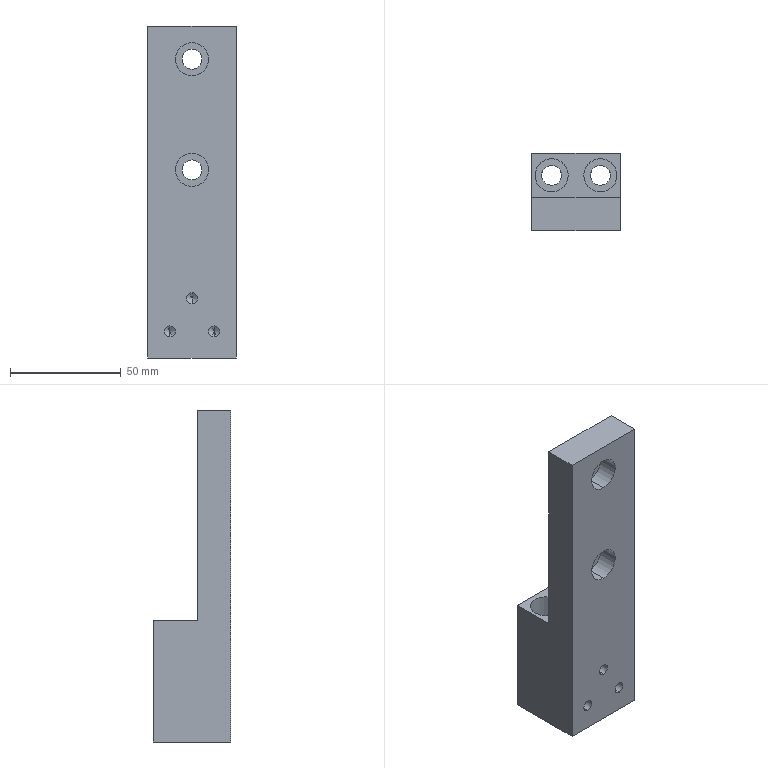Part | SolidWorks | features BaseBody 1 | 1 solid | 52 faces | box 40 x 35 x 150 mm | volume 115005 mm3 | cylinder 28 | cone 12 | plane 12 | commonest cylinder face diameters 9 x8 15 x8 5 x6 6.8 x6
STEP:
#1=CARTESIAN_POINT('',(0.,17.,-45.5));
#2=VERTEX_POINT('',#1);
#3=CARTESIAN_POINT('',(0.,17.,-50.5));
#4=VERTEX_POINT('',#3);
#5=CARTESIAN_POINT('',(0.,17.,-48.));
#6=DIRECTION('',(0.,-1.,0.));
#7=DIRECTION('',(0.,0.,-1.));
#8=AXIS2_PLACEMENT_3D('',#5,#6,#7);
#9=CIRCLE('',#8,2.5);
#10=EDGE_CURVE('',#2,#4,#9,.T.);
#11=ORIENTED_EDGE('',*,*,#10,.F.);
#12=CARTESIAN_POINT('',(0.,0.,-45.5));
#13=VERTEX_POINT('',#12);
#14=CARTESIAN_POINT('',(0.,0.,-45.5));
#15=DIRECTION('',(0.,-1.,0.));
#16=VECTOR('',#15,1000.);
#17=LINE('',#14,#16);
#18=EDGE_CURVE('',#2,#13,#17,.T.);
#19=ORIENTED_EDGE('',*,*,#18,.T.);
#20=CARTESIAN_POINT('',(0.,0.,-50.5));
#21=VERTEX_POINT('',#20);
#22=CARTESIAN_POINT('',(0.,0.,-48.));
#23=DIRECTION('',(0.,-1.,0.));
#24=DIRECTION('',(0.,0.,-1.));
#25=AXIS2_PLACEMENT_3D('',#22,#23,#24);
#26=CIRCLE('',#25,2.5);
#27=EDGE_CURVE('',#13,#21,#26,.T.);
#28=ORIENTED_EDGE('',*,*,#27,.T.);
#29=CARTESIAN_POINT('',(0.,0.,-50.5));
#30=DIRECTION('',(0.,-1.,0.));
#31=VECTOR('',#30,1000.);
#32=LINE('',#29,#31);
#33=EDGE_CURVE('',#4,#21,#32,.T.);
#34=ORIENTED_EDGE('',*,*,#33,.F.);
#35=EDGE_LOOP('',(#11,#19,#28,#34));
#36=FACE_OUTER_BOUND('',#35,.T.);
#37=CARTESIAN_POINT('',(0.,0.,-48.));
#38=DIRECTION('',(0.,-1.,0.));
#39=DIRECTION('',(0.,0.,-1.));
#40=AXIS2_PLACEMENT_3D('',#37,#38,#39);
#41=CYLINDRICAL_SURFACE('',#40,2.5);
#42=ADVANCED_FACE('',(#36),#41,.F.);
#43=CARTESIAN_POINT('',(0.,18.502,-48.));
#44=VERTEX_POINT('',#43);
#45=CARTESIAN_POINT('',(0.,17.,-50.5));
#46=DIRECTION('',(0.,-0.515,-0.8572));
#47=VECTOR('',#46,1000.);
#48=LINE('',#45,#47);
#49=EDGE_CURVE('',#44,#4,#48,.T.);
#50=ORIENTED_EDGE('',*,*,#49,.F.);
#51=CARTESIAN_POINT('',(0.,17.,-45.5));
#52=DIRECTION('',(0.,-0.515,0.8572));
#53=VECTOR('',#52,1000.);
#54=LINE('',#51,#53);
#55=EDGE_CURVE('',#44,#2,#54,.T.);
#56=ORIENTED_EDGE('',*,*,#55,.T.);
#57=ORIENTED_EDGE('',*,*,#10,.T.);
#58=EDGE_LOOP('',(#50,#56,#57));
#59=FACE_OUTER_BOUND('',#58,.T.);
#60=CARTESIAN_POINT('',(0.,17.,-48.));
#61=DIRECTION('',(0.,-1.,0.));
#62=DIRECTION('',(0.,0.,-1.));
#63=AXIS2_PLACEMENT_3D('',#60,#61,#62);
#64=CONICAL_SURFACE('',#63,2.5,1.03);
#65=ADVANCED_FACE('',(#59),#64,.F.);
#66=CARTESIAN_POINT('',(-10.,17.,-60.5));
#67=VERTEX_POINT('',#66);
#68=CARTESIAN_POINT('',(-10.,17.,-65.5));
#69=VERTEX_POINT('',#68);
#70=CARTESIAN_POINT('',(-10.,17.,-63.));
#71=DIRECTION('',(0.,-1.,0.));
#72=DIRECTION('',(0.,0.,-1.));
#73=AXIS2_PLACEMENT_3D('',#70,#71,#72);
#74=CIRCLE('',#73,2.5);
#75=EDGE_CURVE('',#67,#69,#74,.T.);
#76=ORIENTED_EDGE('',*,*,#75,.F.);
#77=CARTESIAN_POINT('',(-10.,0.,-60.5));
#78=VERTEX_POINT('',#77);
#79=CARTESIAN_POINT('',(-10.,0.,-60.5));
#80=DIRECTION('',(0.,-1.,0.));
#81=VECTOR('',#80,1000.);
#82=LINE('',#79,#81);
#83=EDGE_CURVE('',#67,#78,#82,.T.);
#84=ORIENTED_EDGE('',*,*,#83,.T.);
#85=CARTESIAN_POINT('',(-10.,0.,-65.5));
#86=VERTEX_POINT('',#85);
#87=CARTESIAN_POINT('',(-10.,0.,-63.));
#88=DIRECTION('',(0.,-1.,0.));
#89=DIRECTION('',(0.,0.,-1.));
#90=AXIS2_PLACEMENT_3D('',#87,#88,#89);
#91=CIRCLE('',#90,2.5);
#92=EDGE_CURVE('',#78,#86,#91,.T.);
#93=ORIENTED_EDGE('',*,*,#92,.T.);
#94=CARTESIAN_POINT('',(-10.,0.,-65.5));
#95=DIRECTION('',(0.,-1.,0.));
#96=VECTOR('',#95,1000.);
#97=LINE('',#94,#96);
#98=EDGE_CURVE('',#69,#86,#97,.T.);
#99=ORIENTED_EDGE('',*,*,#98,.F.);
#100=EDGE_LOOP('',(#76,#84,#93,#99));
#101=FACE_OUTER_BOUND('',#100,.T.);
#102=CARTESIAN_POINT('',(-10.,0.,-63.));
#103=DIRECTION('',(0.,-1.,0.));
#104=DIRECTION('',(0.,0.,-1.));
#105=AXIS2_PLACEMENT_3D('',#102,#103,#104);
#106=CYLINDRICAL_SURFACE('',#105,2.5);
#107=ADVANCED_FACE('',(#101),#106,.F.);
#108=CARTESIAN_POINT('',(-10.,18.502,-63.));
#109=VERTEX_POINT('',#108);
#110=CARTESIAN_POINT('',(-10.,17.,-65.5));
#111=DIRECTION('',(0.,-0.515,-0.8572));
#112=VECTOR('',#111,1000.);
#113=LINE('',#110,#112);
#114=EDGE_CURVE('',#109,#69,#113,.T.);
#115=ORIENTED_EDGE('',*,*,#114,.F.);
#116=CARTESIAN_POINT('',(-10.,17.,-60.5));
#117=DIRECTION('',(0.,-0.515,0.8572));
#118=VECTOR('',#117,1000.);
#119=LINE('',#116,#118);
#120=EDGE_CURVE('',#109,#67,#119,.T.);
#121=ORIENTED_EDGE('',*,*,#120,.T.);
#122=ORIENTED_EDGE('',*,*,#75,.T.);
#123=EDGE_LOOP('',(#115,#121,#122));
#124=FACE_OUTER_BOUND('',#123,.T.);
#125=CARTESIAN_POINT('',(-10.,17.,-63.));
#126=DIRECTION('',(0.,-1.,0.));
#127=DIRECTION('',(0.,0.,-1.));
#128=AXIS2_PLACEMENT_3D('',#125,#126,#127);
#129=CONICAL_SURFACE('',#128,2.5,1.03);
#130=ADVANCED_FACE('',(#124),#129,.F.);
#131=CARTESIAN_POINT('',(10.,17.,-60.5));
#132=VERTEX_POINT('',#131);
#133=CARTESIAN_POINT('',(10.,17.,-65.5));
#134=VERTEX_POINT('',#133);
#135=CARTESIAN_POINT('',(10.,17.,-63.));
#136=DIRECTION('',(0.,-1.,0.));
#137=DIRECTION('',(0.,0.,-1.));
#138=AXIS2_PLACEMENT_3D('',#135,#136,#137);
#139=CIRCLE('',#138,2.5);
#140=EDGE_CURVE('',#132,#134,#139,.T.);
#141=ORIENTED_EDGE('',*,*,#140,.F.);
#142=CARTESIAN_POINT('',(10.,0.,-60.5));
#143=VERTEX_POINT('',#142);
#144=CARTESIAN_POINT('',(10.,0.,-60.5));
#145=DIRECTION('',(0.,-1.,0.));
#146=VECTOR('',#145,1000.);
#147=LINE('',#144,#146);
#148=EDGE_CURVE('',#132,#143,#147,.T.);
#149=ORIENTED_EDGE('',*,*,#148,.T.);
#150=CARTESIAN_POINT('',(10.,0.,-65.5));
#151=VERTEX_POINT('',#150);
#152=CARTESIAN_POINT('',(10.,0.,-63.));
#153=DIRECTION('',(0.,-1.,0.));
#154=DIRECTION('',(0.,0.,-1.));
#155=AXIS2_PLACEMENT_3D('',#152,#153,#154);
#156=CIRCLE('',#155,2.5);
#157=EDGE_CURVE('',#143,#151,#156,.T.);
#158=ORIENTED_EDGE('',*,*,#157,.T.);
#159=CARTESIAN_POINT('',(10.,0.,-65.5));
#160=DIRECTION('',(0.,-1.,0.));
#161=VECTOR('',#160,1000.);
#162=LINE('',#159,#161);
#163=EDGE_CURVE('',#134,#151,#162,.T.);
#164=ORIENTED_EDGE('',*,*,#163,.F.);
#165=EDGE_LOOP('',(#141,#149,#158,#164));
#166=FACE_OUTER_BOUND('',#165,.T.);
#167=CARTESIAN_POINT('',(10.,0.,-63.));
#168=DIRECTION('',(0.,-1.,0.));
#169=DIRECTION('',(0.,0.,-1.));
#170=AXIS2_PLACEMENT_3D('',#167,#168,#169);
#171=CYLINDRICAL_SURFACE('',#170,2.5);
#172=ADVANCED_FACE('',(#166),#171,.F.);
#173=CARTESIAN_POINT('',(10.,18.502,-63.));
#174=VERTEX_POINT('',#173);
#175=CARTESIAN_POINT('',(10.,17.,-65.5));
#176=DIRECTION('',(0.,-0.515,-0.8572));
#177=VECTOR('',#176,1000.);
#178=LINE('',#175,#177);
#179=EDGE_CURVE('',#174,#134,#178,.T.);
#180=ORIENTED_EDGE('',*,*,#179,.F.);
#181=CARTESIAN_POINT('',(10.,17.,-60.5));
#182=DIRECTION('',(0.,-0.515,0.8572));
#183=VECTOR('',#182,1000.);
#184=LINE('',#181,#183);
#185=EDGE_CURVE('',#174,#132,#184,.T.);
#186=ORIENTED_EDGE('',*,*,#185,.T.);
#187=ORIENTED_EDGE('',*,*,#140,.T.);
#188=EDGE_LOOP('',(#180,#186,#187));
#189=FACE_OUTER_BOUND('',#188,.T.);
#190=CARTESIAN_POINT('',(10.,17.,-63.));
#191=DIRECTION('',(0.,-1.,0.));
#192=DIRECTION('',(0.,0.,-1.));
#193=AXIS2_PLACEMENT_3D('',#190,#191,#192);
#194=CONICAL_SURFACE('',#193,2.5,1.03);
#195=ADVANCED_FACE('',(#189),#194,.F.);
#196=CARTESIAN_POINT('',(-2.25,7.5,-51.6));
#197=VERTEX_POINT('',#196);
#198=CARTESIAN_POINT('',(-2.25,7.5,-58.4));
#199=VERTEX_POINT('',#198);
#200=CARTESIAN_POINT('',(-2.25,7.5,-55.));
#201=DIRECTION('',(1.,0.,0.));
#202=DIRECTION('',(0.,0.,-1.));
#203=AXIS2_PLACEMENT_3D('',#200,#201,#202);
#204=CIRCLE('',#203,3.4);
#205=EDGE_CURVE('',#197,#199,#204,.T.);
#206=ORIENTED_EDGE('',*,*,#205,.F.);
#207=CARTESIAN_POINT('',(20.,7.5,-51.6));
#208=VERTEX_POINT('',#207);
#209=CARTESIAN_POINT('',(20.,7.5,-51.6));
#210=DIRECTION('',(1.,0.,0.));
#211=VECTOR('',#210,1000.);
#212=LINE('',#209,#211);
#213=EDGE_CURVE('',#197,#208,#212,.T.);
#214=ORIENTED_EDGE('',*,*,#213,.T.);
#215=CARTESIAN_POINT('',(20.,7.5,-58.4));
#216=VERTEX_POINT('',#215);
#217=CARTESIAN_POINT('',(20.,7.5,-55.));
#218=DIRECTION('',(1.,0.,0.));
#219=DIRECTION('',(0.,0.,-1.));
#220=AXIS2_PLACEMENT_3D('',#217,#218,#219);
#221=CIRCLE('',#220,3.4);
#222=EDGE_CURVE('',#208,#216,#221,.T.);
#223=ORIENTED_EDGE('',*,*,#222,.T.);
#224=CARTESIAN_POINT('',(20.,7.5,-58.4));
#225=DIRECTION('',(1.,0.,0.));
#226=VECTOR('',#225,1000.);
#227=LINE('',#224,#226);
#228=EDGE_CURVE('',#199,#216,#227,.T.);
#229=ORIENTED_EDGE('',*,*,#228,.F.);
#230=EDGE_LOOP('',(#206,#214,#223,#229));
#231=FACE_OUTER_BOUND('',#230,.T.);
#232=CARTESIAN_POINT('',(20.,7.5,-55.));
#233=DIRECTION('',(1.,0.,0.));
#234=DIRECTION('',(0.,0.,-1.));
#235=AXIS2_PLACEMENT_3D('',#232,#233,#234);
#236=CYLINDRICAL_SURFACE('',#235,3.4);
#237=ADVANCED_FACE('',(#231),#236,.F.);
#238=CARTESIAN_POINT('',(-4.293,7.5,-55.));
#239=VERTEX_POINT('',#238);
#240=CARTESIAN_POINT('',(-2.25,7.5,-58.4));
#241=DIRECTION('',(0.515,0.,-0.8572));
#242=VECTOR('',#241,1000.);
#243=LINE('',#240,#242);
#244=EDGE_CURVE('',#239,#199,#243,.T.);
#245=ORIENTED_EDGE('',*,*,#244,.F.);
#246=CARTESIAN_POINT('',(-2.25,7.5,-51.6));
#247=DIRECTION('',(0.515,0.,0.8572));
#248=VECTOR('',#247,1000.);
#249=LINE('',#246,#248);
#250=EDGE_CURVE('',#239,#197,#249,.T.);
#251=ORIENTED_EDGE('',*,*,#250,.T.);
#252=ORIENTED_EDGE('',*,*,#205,.T.);
#253=EDGE_LOOP('',(#245,#251,#252));
#254=FACE_OUTER_BOUND('',#253,.T.);
#255=CARTESIAN_POINT('',(-2.25,7.5,-55.));
#256=DIRECTION('',(1.,0.,0.));
#257=DIRECTION('',(0.,0.,-1.));
#258=AXIS2_PLACEMENT_3D('',#255,#256,#257);
#259=CONICAL_SURFACE('',#258,3.4,1.03);
#260=ADVANCED_FACE('',(#254),#259,.F.);
#261=CARTESIAN_POINT('',(-2.25,7.5,-11.6));
#262=VERTEX_POINT('',#261);
#263=CARTESIAN_POINT('',(-2.25,7.5,-18.4));
#264=VERTEX_POINT('',#263);
#265=CARTESIAN_POINT('',(-2.25,7.5,-15.));
#266=DIRECTION('',(1.,0.,0.));
#267=DIRECTION('',(0.,0.,-1.));
#268=AXIS2_PLACEMENT_3D('',#265,#266,#267);
#269=CIRCLE('',#268,3.4);
#270=EDGE_CURVE('',#262,#264,#269,.T.);
#271=ORIENTED_EDGE('',*,*,#270,.F.);
#272=CARTESIAN_POINT('',(20.,7.5,-11.6));
#273=VERTEX_POINT('',#272);
#274=CARTESIAN_POINT('',(20.,7.5,-11.6));
#275=DIRECTION('',(1.,0.,0.));
#276=VECTOR('',#275,1000.);
#277=LINE('',#274,#276);
#278=EDGE_CURVE('',#262,#273,#277,.T.);
#279=ORIENTED_EDGE('',*,*,#278,.T.);
#280=CARTESIAN_POINT('',(20.,7.5,-18.4));
#281=VERTEX_POINT('',#280);
#282=CARTESIAN_POINT('',(20.,7.5,-15.));
#283=DIRECTION('',(1.,0.,0.));
#284=DIRECTION('',(0.,0.,-1.));
#285=AXIS2_PLACEMENT_3D('',#282,#283,#284);
#286=CIRCLE('',#285,3.4);
#287=EDGE_CURVE('',#273,#281,#286,.T.);
#288=ORIENTED_EDGE('',*,*,#287,.T.);
#289=CARTESIAN_POINT('',(20.,7.5,-18.4));
#290=DIRECTION('',(1.,0.,0.));
#291=VECTOR('',#290,1000.);
#292=LINE('',#289,#291);
#293=EDGE_CURVE('',#264,#281,#292,.T.);
#294=ORIENTED_EDGE('',*,*,#293,.F.);
#295=EDGE_LOOP('',(#271,#279,#288,#294));
#296=FACE_OUTER_BOUND('',#295,.T.);
#297=CARTESIAN_POINT('',(20.,7.5,-15.));
#298=DIRECTION('',(1.,0.,0.));
#299=DIRECTION('',(0.,0.,-1.));
#300=AXIS2_PLACEMENT_3D('',#297,#298,#299);
#301=CYLINDRICAL_SURFACE('',#300,3.4);
#302=ADVANCED_FACE('',(#296),#301,.F.);
#303=CARTESIAN_POINT('',(-4.293,7.5,-15.));
#304=VERTEX_POINT('',#303);
#305=CARTESIAN_POINT('',(-2.25,7.5,-18.4));
#306=DIRECTION('',(0.515,0.,-0.8572));
#307=VECTOR('',#306,1000.);
#308=LINE('',#305,#307);
#309=EDGE_CURVE('',#304,#264,#308,.T.);
#310=ORIENTED_EDGE('',*,*,#309,.F.);
#311=CARTESIAN_POINT('',(-2.25,7.5,-11.6));
#312=DIRECTION('',(0.515,0.,0.8572));
#313=VECTOR('',#312,1000.);
#314=LINE('',#311,#313);
#315=EDGE_CURVE('',#304,#262,#314,.T.);
#316=ORIENTED_EDGE('',*,*,#315,.T.);
#317=ORIENTED_EDGE('',*,*,#270,.T.);
#318=EDGE_LOOP('',(#310,#316,#317));
#319=FACE_OUTER_BOUND('',#318,.T.);
#320=CARTESIAN_POINT('',(-2.25,7.5,-15.));
#321=DIRECTION('',(1.,0.,0.));
#322=DIRECTION('',(0.,0.,-1.));
#323=AXIS2_PLACEMENT_3D('',#320,#321,#322);
#324=CONICAL_SURFACE('',#323,3.4,1.03);
#325=ADVANCED_FACE('',(#319),#324,.F.);
#326=CARTESIAN_POINT('',(-2.25,7.5,28.4));
#327=VERTEX_POINT('',#326);
#328=CARTESIAN_POINT('',(-2.25,7.5,21.6));
#329=VERTEX_POINT('',#328);
#330=CARTESIAN_POINT('',(-2.25,7.5,25.));
#331=DIRECTION('',(1.,0.,0.));
#332=DIRECTION('',(0.,0.,-1.));
#333=AXIS2_PLACEMENT_3D('',#330,#331,#332);
#334=CIRCLE('',#333,3.4);
#335=EDGE_CURVE('',#327,#329,#334,.T.);
#336=ORIENTED_EDGE('',*,*,#335,.F.);
#337=CARTESIAN_POINT('',(20.,7.5,28.4));
#338=VERTEX_POINT('',#337);
#339=CARTESIAN_POINT('',(20.,7.5,28.4));
#340=DIRECTION('',(1.,0.,0.));
#341=VECTOR('',#340,1000.);
#342=LINE('',#339,#341);
#343=EDGE_CURVE('',#327,#338,#342,.T.);
#344=ORIENTED_EDGE('',*,*,#343,.T.);
#345=CARTESIAN_POINT('',(20.,7.5,21.6));
#346=VERTEX_POINT('',#345);
#347=CARTESIAN_POINT('',(20.,7.5,25.));
#348=DIRECTION('',(1.,0.,0.));
#349=DIRECTION('',(0.,0.,-1.));
#350=AXIS2_PLACEMENT_3D('',#347,#348,#349);
#351=CIRCLE('',#350,3.4);
#352=EDGE_CURVE('',#338,#346,#351,.T.);
#353=ORIENTED_EDGE('',*,*,#352,.T.);
#354=CARTESIAN_POINT('',(20.,7.5,21.6));
#355=DIRECTION('',(1.,0.,0.));
#356=VECTOR('',#355,1000.);
#357=LINE('',#354,#356);
#358=EDGE_CURVE('',#329,#346,#357,.T.);
#359=ORIENTED_EDGE('',*,*,#358,.F.);
#360=EDGE_LOOP('',(#336,#344,#353,#359));
#361=FACE_OUTER_BOUND('',#360,.T.);
#362=CARTESIAN_POINT('',(20.,7.5,25.));
#363=DIRECTION('',(1.,0.,0.));
#364=DIRECTION('',(0.,0.,-1.));
#365=AXIS2_PLACEMENT_3D('',#362,#363,#364);
#366=CYLINDRICAL_SURFACE('',#365,3.4);
#367=ADVANCED_FACE('',(#361),#366,.F.);
#368=CARTESIAN_POINT('',(-4.293,7.5,25.));
#369=VERTEX_POINT('',#368);
#370=CARTESIAN_POINT('',(-2.25,7.5,21.6));
#371=DIRECTION('',(0.515,0.,-0.8572));
#372=VECTOR('',#371,1000.);
#373=LINE('',#370,#372);
#374=EDGE_CURVE('',#369,#329,#373,.T.);
#375=ORIENTED_EDGE('',*,*,#374,.F.);
#376=CARTESIAN_POINT('',(-2.25,7.5,28.4));
#377=DIRECTION('',(0.515,0.,0.8572));
#378=VECTOR('',#377,1000.);
#379=LINE('',#376,#378);
#380=EDGE_CURVE('',#369,#327,#379,.T.);
#381=ORIENTED_EDGE('',*,*,#380,.T.);
#382=ORIENTED_EDGE('',*,*,#335,.T.);
#383=EDGE_LOOP('',(#375,#381,#382));
#384=FACE_OUTER_BOUND('',#383,.T.);
#385=CARTESIAN_POINT('',(-2.25,7.5,25.));
#386=DIRECTION('',(1.,0.,0.));
#387=DIRECTION('',(0.,0.,-1.));
#388=AXIS2_PLACEMENT_3D('',#385,#386,#387);
#389=CONICAL_SURFACE('',#388,3.4,1.03);
#390=ADVANCED_FACE('',(#384),#389,.F.);
#391=CARTESIAN_POINT('',(3.5,25.,-40.));
#392=VERTEX_POINT('',#391);
#393=CARTESIAN_POINT('',(18.5,25.,-40.));
#394=VERTEX_POINT('',#393);
#395=CARTESIAN_POINT('',(11.,25.,-40.));
#396=DIRECTION('',(0.,0.,1.));
#397=DIRECTION('',(1.,0.,0.));
#398=AXIS2_PLACEMENT_3D('',#395,#396,#397);
#399=CIRCLE('',#398,7.5);
#400=EDGE_CURVE('',#392,#394,#399,.T.);
#401=ORIENTED_EDGE('',*,*,#400,.F.);
#402=CARTESIAN_POINT('',(3.5,25.,-20.));
#403=VERTEX_POINT('',#402);
#404=CARTESIAN_POINT('',(3.5,25.,-20.));
#405=DIRECTION('',(0.,0.,1.));
#406=VECTOR('',#405,1000.);
#407=LINE('',#404,#406);
#408=EDGE_CURVE('',#392,#403,#407,.T.);
#409=ORIENTED_EDGE('',*,*,#408,.T.);
#410=CARTESIAN_POINT('',(18.5,25.,-20.));
#411=VERTEX_POINT('',#410);
#412=CARTESIAN_POINT('',(11.,25.,-20.));
#413=DIRECTION('',(0.,0.,1.));
#414=DIRECTION('',(1.,0.,0.));
#415=AXIS2_PLACEMENT_3D('',#412,#413,#414);
#416=CIRCLE('',#415,7.5);
#417=EDGE_CURVE('',#403,#411,#416,.T.);
#418=ORIENTED_EDGE('',*,*,#417,.T.);
#419=CARTESIAN_POINT('',(18.5,25.,-20.));
#420=DIRECTION('',(0.,0.,1.));
#421=VECTOR('',#420,1000.);
#422=LINE('',#419,#421);
#423=EDGE_CURVE('',#394,#411,#422,.T.);
#424=ORIENTED_EDGE('',*,*,#423,.F.);
#425=EDGE_LOOP('',(#401,#409,#418,#424));
#426=FACE_OUTER_BOUND('',#425,.T.);
#427=CARTESIAN_POINT('',(11.,25.,-20.));
#428=DIRECTION('',(0.,0.,1.));
#429=DIRECTION('',(1.,0.,0.));
#430=AXIS2_PLACEMENT_3D('',#427,#428,#429);
#431=CYLINDRICAL_SURFACE('',#430,7.5);
#432=ADVANCED_FACE('',(#426),#431,.F.);
#433=CARTESIAN_POINT('',(6.5,25.,-75.));
#434=VERTEX_POINT('',#433);
#435=CARTESIAN_POINT('',(15.5,25.,-75.));
#436=VERTEX_POINT('',#435);
#437=CARTESIAN_POINT('',(11.,25.,-75.));
#438=DIRECTION('',(0.,0.,1.));
#439=DIRECTION('',(1.,0.,0.));
#440=AXIS2_PLACEMENT_3D('',#437,#438,#439);
#441=CIRCLE('',#440,4.5);
#442=EDGE_CURVE('',#434,#436,#441,.T.);
#443=ORIENTED_EDGE('',*,*,#442,.F.);
#444=CARTESIAN_POINT('',(6.5,25.,-40.));
#445=VERTEX_POINT('',#444);
#446=CARTESIAN_POINT('',(6.5,25.,-20.));
#447=DIRECTION('',(0.,0.,1.));
#448=VECTOR('',#447,1000.);
#449=LINE('',#446,#448);
#450=EDGE_CURVE('',#434,#445,#449,.T.);
#451=ORIENTED_EDGE('',*,*,#450,.T.);
#452=CARTESIAN_POINT('',(15.5,25.,-40.));
#453=VERTEX_POINT('',#452);
#454=CARTESIAN_POINT('',(11.,25.,-40.));
#455=DIRECTION('',(0.,0.,1.));
#456=DIRECTION('',(1.,0.,0.));
#457=AXIS2_PLACEMENT_3D('',#454,#455,#456);
#458=CIRCLE('',#457,4.5);
#459=EDGE_CURVE('',#445,#453,#458,.T.);
#460=ORIENTED_EDGE('',*,*,#459,.T.);
#461=CARTESIAN_POINT('',(15.5,25.,-20.));
#462=DIRECTION('',(0.,0.,1.));
#463=VECTOR('',#462,1000.);
#464=LINE('',#461,#463);
#465=EDGE_CURVE('',#436,#453,#464,.T.);
#466=ORIENTED_EDGE('',*,*,#465,.F.);
#467=EDGE_LOOP('',(#443,#451,#460,#466));
#468=FACE_OUTER_BOUND('',#467,.T.);
#469=CARTESIAN_POINT('',(11.,25.,-20.));
#470=DIRECTION('',(0.,0.,1.));
#471=DIRECTION('',(1.,0.,0.));
#472=AXIS2_PLACEMENT_3D('',#469,#470,#471);
#473=CYLINDRICAL_SURFACE('',#472,4.5);
#474=ADVANCED_FACE('',(#468),#473,.F.);
#475=CARTESIAN_POINT('',(-18.5,25.,-40.));
#476=VERTEX_POINT('',#475);
#477=CARTESIAN_POINT('',(-3.5,25.,-40.));
#478=VERTEX_POINT('',#477);
#479=CARTESIAN_POINT('',(-11.,25.,-40.));
#480=DIRECTION('',(0.,0.,1.));
#481=DIRECTION('',(1.,0.,0.));
#482=AXIS2_PLACEMENT_3D('',#479,#480,#481);
#483=CIRCLE('',#482,7.5);
#484=EDGE_CURVE('',#476,#478,#483,.T.);
#485=ORIENTED_EDGE('',*,*,#484,.F.);
#486=CARTESIAN_POINT('',(-18.5,25.,-20.));
#487=VERTEX_POINT('',#486);
#488=CARTESIAN_POINT('',(-18.5,25.,-20.));
#489=DIRECTION('',(0.,0.,1.));
#490=VECTOR('',#489,1000.);
#491=LINE('',#488,#490);
#492=EDGE_CURVE('',#476,#487,#491,.T.);
#493=ORIENTED_EDGE('',*,*,#492,.T.);
#494=CARTESIAN_POINT('',(-3.5,25.,-20.));
#495=VERTEX_POINT('',#494);
#496=CARTESIAN_POINT('',(-11.,25.,-20.));
#497=DIRECTION('',(0.,0.,1.));
#498=DIRECTION('',(1.,0.,0.));
#499=AXIS2_PLACEMENT_3D('',#496,#497,#498);
#500=CIRCLE('',#499,7.5);
#501=EDGE_CURVE('',#487,#495,#500,.T.);
#502=ORIENTED_EDGE('',*,*,#501,.T.);
#503=CARTESIAN_POINT('',(-3.5,25.,-20.));
#504=DIRECTION('',(0.,0.,1.));
#505=VECTOR('',#504,1000.);
#506=LINE('',#503,#505);
#507=EDGE_CURVE('',#478,#495,#506,.T.);
#508=ORIENTED_EDGE('',*,*,#507,.F.);
#509=EDGE_LOOP('',(#485,#493,#502,#508));
#510=FACE_OUTER_BOUND('',#509,.T.);
#511=CARTESIAN_POINT('',(-11.,25.,-20.));
#512=DIRECTION('',(0.,0.,1.));
#513=DIRECTION('',(1.,0.,0.));
#514=AXIS2_PLACEMENT_3D('',#511,#512,#513);
#515=CYLINDRICAL_SURFACE('',#514,7.5);
#516=ADVANCED_FACE('',(#510),#515,.F.);
#517=CARTESIAN_POINT('',(-15.5,25.,-75.));
#518=VERTEX_POINT('',#517);
#519=CARTESIAN_POINT('',(-6.5,25.,-75.));
#520=VERTEX_POINT('',#519);
#521=CARTESIAN_POINT('',(-11.,25.,-75.));
#522=DIRECTION('',(0.,0.,1.));
#523=DIRECTION('',(1.,0.,0.));
#524=AXIS2_PLACEMENT_3D('',#521,#522,#523);
#525=CIRCLE('',#524,4.5);
#526=EDGE_CURVE('',#518,#520,#525,.T.);
#527=ORIENTED_EDGE('',*,*,#526,.F.);
#528=CARTESIAN_POINT('',(-15.5,25.,-40.));
#529=VERTEX_POINT('',#528);
#530=CARTESIAN_POINT('',(-15.5,25.,-20.));
#531=DIRECTION('',(0.,0.,1.));
#532=VECTOR('',#531,1000.);
#533=LINE('',#530,#532);
#534=EDGE_CURVE('',#518,#529,#533,.T.);
#535=ORIENTED_EDGE('',*,*,#534,.T.);
#536=CARTESIAN_POINT('',(-6.5,25.,-40.));
#537=VERTEX_POINT('',#536);
#538=CARTESIAN_POINT('',(-11.,25.,-40.));
#539=DIRECTION('',(0.,0.,1.));
#540=DIRECTION('',(1.,0.,0.));
#541=AXIS2_PLACEMENT_3D('',#538,#539,#540);
#542=CIRCLE('',#541,4.5);
#543=EDGE_CURVE('',#529,#537,#542,.T.);
#544=ORIENTED_EDGE('',*,*,#543,.T.);
#545=CARTESIAN_POINT('',(-6.5,25.,-20.));
#546=DIRECTION('',(0.,0.,1.));
#547=VECTOR('',#546,1000.);
#548=LINE('',#545,#547);
#549=EDGE_CURVE('',#520,#537,#548,.T.);
#550=ORIENTED_EDGE('',*,*,#549,.F.);
#551=EDGE_LOOP('',(#527,#535,#544,#550));
#552=FACE_OUTER_BOUND('',#551,.T.);
#553=CARTESIAN_POINT('',(-11.,25.,-20.));
#554=DIRECTION('',(0.,0.,1.));
#555=DIRECTION('',(1.,0.,0.));
#556=AXIS2_PLACEMENT_3D('',#553,#554,#555);
#557=CYLINDRICAL_SURFACE('',#556,4.5);
#558=ADVANCED_FACE('',(#552),#557,.F.);
#559=CARTESIAN_POINT('',(0.,9.,67.5));
#560=VERTEX_POINT('',#559);
#561=CARTESIAN_POINT('',(0.,9.,52.5));
#562=VERTEX_POINT('',#561);
#563=CARTESIAN_POINT('',(0.,9.,60.));
#564=DIRECTION('',(0.,-1.,0.));
#565=DIRECTION('',(0.,0.,-1.));
#566=AXIS2_PLACEMENT_3D('',#563,#564,#565);
#567=CIRCLE('',#566,7.5);
#568=EDGE_CURVE('',#560,#562,#567,.T.);
#569=ORIENTED_EDGE('',*,*,#568,.F.);
#570=CARTESIAN_POINT('',(0.,0.,67.5));
#571=VERTEX_POINT('',#570);
#572=CARTESIAN_POINT('',(0.,0.,67.5));
#573=DIRECTION('',(0.,-1.,0.));
#574=VECTOR('',#573,1000.);
#575=LINE('',#572,#574);
#576=EDGE_CURVE('',#560,#571,#575,.T.);
#577=ORIENTED_EDGE('',*,*,#576,.T.);
#578=CARTESIAN_POINT('',(0.,0.,52.5));
#579=VERTEX_POINT('',#578);
#580=CARTESIAN_POINT('',(0.,0.,60.));
#581=DIRECTION('',(0.,-1.,0.));
#582=DIRECTION('',(0.,0.,-1.));
#583=AXIS2_PLACEMENT_3D('',#580,#581,#582);
#584=CIRCLE('',#583,7.5);
#585=EDGE_CURVE('',#571,#579,#584,.T.);
#586=ORIENTED_EDGE('',*,*,#585,.T.);
#587=CARTESIAN_POINT('',(0.,0.,52.5));
#588=DIRECTION('',(0.,-1.,0.));
#589=VECTOR('',#588,1000.);
#590=LINE('',#587,#589);
#591=EDGE_CURVE('',#562,#579,#590,.T.);
#592=ORIENTED_EDGE('',*,*,#591,.F.);
#593=EDGE_LOOP('',(#569,#577,#586,#592));
#594=FACE_OUTER_BOUND('',#593,.T.);
#595=CARTESIAN_POINT('',(0.,0.,60.));
#596=DIRECTION('',(0.,-1.,0.));
#597=DIRECTION('',(0.,0.,-1.));
#598=AXIS2_PLACEMENT_3D('',#595,#596,#597);
#599=CYLINDRICAL_SURFACE('',#598,7.5);
#600=ADVANCED_FACE('',(#594),#599,.F.);
#601=CARTESIAN_POINT('',(0.,15.,64.5));
#602=VERTEX_POINT('',#601);
#603=CARTESIAN_POINT('',(0.,15.,55.5));
#604=VERTEX_POINT('',#603);
#605=CARTESIAN_POINT('',(0.,15.,60.));
#606=DIRECTION('',(0.,-1.,0.));
#607=DIRECTION('',(0.,0.,-1.));
#608=AXIS2_PLACEMENT_3D('',#605,#606,#607);
#609=CIRCLE('',#608,4.5);
#610=EDGE_CURVE('',#602,#604,#609,.T.);
#611=ORIENTED_EDGE('',*,*,#610,.F.);
#612=CARTESIAN_POINT('',(0.,9.,64.5));
#613=VERTEX_POINT('',#612);
#614=CARTESIAN_POINT('',(0.,0.,64.5));
#615=DIRECTION('',(0.,-1.,0.));
#616=VECTOR('',#615,1000.);
#617=LINE('',#614,#616);
#618=EDGE_CURVE('',#602,#613,#617,.T.);
#619=ORIENTED_EDGE('',*,*,#618,.T.);
#620=CARTESIAN_POINT('',(0.,9.,55.5));
#621=VERTEX_POINT('',#620);
#622=CARTESIAN_POINT('',(0.,9.,60.));
#623=DIRECTION('',(0.,-1.,0.));
#624=DIRECTION('',(0.,0.,-1.));
#625=AXIS2_PLACEMENT_3D('',#622,#623,#624);
#626=CIRCLE('',#625,4.5);
#627=EDGE_CURVE('',#613,#621,#626,.T.);
#628=ORIENTED_EDGE('',*,*,#627,.T.);
#629=CARTESIAN_POINT('',(0.,0.,55.5));
#630=DIRECTION('',(0.,-1.,0.));
#631=VECTOR('',#630,1000.);
#632=LINE('',#629,#631);
#633=EDGE_CURVE('',#604,#621,#632,.T.);
#634=ORIENTED_EDGE('',*,*,#633,.F.);
#635=EDGE_LOOP('',(#611,#619,#628,#634));
#636=FACE_OUTER_BOUND('',#635,.T.);
#637=CARTESIAN_POINT('',(0.,0.,60.));
#638=DIRECTION('',(0.,-1.,0.));
#639=DIRECTION('',(0.,0.,-1.));
#640=AXIS2_PLACEMENT_3D('',#637,#638,#639);
#641=CYLINDRICAL_SURFACE('',#640,4.5);
#642=ADVANCED_FACE('',(#636),#641,.F.);
#643=CARTESIAN_POINT('',(0.,9.,17.5));
#644=VERTEX_POINT('',#643);
#645=CARTESIAN_POINT('',(0.,9.,2.5));
#646=VERTEX_POINT('',#645);
#647=CARTESIAN_POINT('',(0.,9.,10.));
#648=DIRECTION('',(0.,-1.,0.));
#649=DIRECTION('',(0.,0.,-1.));
#650=AXIS2_PLACEMENT_3D('',#647,#648,#649);
#651=CIRCLE('',#650,7.5);
#652=EDGE_CURVE('',#644,#646,#651,.T.);
#653=ORIENTED_EDGE('',*,*,#652,.F.);
#654=CARTESIAN_POINT('',(0.,0.,17.5));
#655=VERTEX_POINT('',#654);
#656=CARTESIAN_POINT('',(0.,0.,17.5));
#657=DIRECTION('',(0.,-1.,0.));
#658=VECTOR('',#657,1000.);
#659=LINE('',#656,#658);
#660=EDGE_CURVE('',#644,#655,#659,.T.);
#661=ORIENTED_EDGE('',*,*,#660,.T.);
#662=CARTESIAN_POINT('',(0.,0.,2.5));
#663=VERTEX_POINT('',#662);
#664=CARTESIAN_POINT('',(0.,0.,10.));
#665=DIRECTION('',(0.,-1.,0.));
#666=DIRECTION('',(0.,0.,-1.));
#667=AXIS2_PLACEMENT_3D('',#664,#665,#666);
#668=CIRCLE('',#667,7.5);
#669=EDGE_CURVE('',#655,#663,#668,.T.);
#670=ORIENTED_EDGE('',*,*,#669,.T.);
#671=CARTESIAN_POINT('',(0.,0.,2.5));
#672=DIRECTION('',(0.,-1.,0.));
#673=VECTOR('',#672,1000.);
#674=LINE('',#671,#673);
#675=EDGE_CURVE('',#646,#663,#674,.T.);
#676=ORIENTED_EDGE('',*,*,#675,.F.);
#677=EDGE_LOOP('',(#653,#661,#670,#676));
#678=FACE_OUTER_BOUND('',#677,.T.);
#679=CARTESIAN_POINT('',(0.,0.,10.));
#680=DIRECTION('',(0.,-1.,0.));
#681=DIRECTION('',(0.,0.,-1.));
#682=AXIS2_PLACEMENT_3D('',#679,#680,#681);
#683=CYLINDRICAL_SURFACE('',#682,7.5);
#684=ADVANCED_FACE('',(#678),#683,.F.);
#685=CARTESIAN_POINT('',(0.,15.,14.5));
#686=VERTEX_POINT('',#685);
#687=CARTESIAN_POINT('',(0.,15.,5.5));
#688=VERTEX_POINT('',#687);
#689=CARTESIAN_POINT('',(0.,15.,10.));
#690=DIRECTION('',(0.,-1.,0.));
#691=DIRECTION('',(0.,0.,-1.));
#692=AXIS2_PLACEMENT_3D('',#689,#690,#691);
#693=CIRCLE('',#692,4.5);
#694=EDGE_CURVE('',#686,#688,#693,.T.);
#695=ORIENTED_EDGE('',*,*,#694,.F.);
#696=CARTESIAN_POINT('',(0.,9.,14.5));
#697=VERTEX_POINT('',#696);
#698=CARTESIAN_POINT('',(0.,0.,14.5));
#699=DIRECTION('',(0.,-1.,0.));
#700=VECTOR('',#699,1000.);
#701=LINE('',#698,#700);
#702=EDGE_CURVE('',#686,#697,#701,.T.);
#703=ORIENTED_EDGE('',*,*,#702,.T.);
#704=CARTESIAN_POINT('',(0.,9.,5.5));
#705=VERTEX_POINT('',#704);
#706=CARTESIAN_POINT('',(0.,9.,10.));
#707=DIRECTION('',(0.,-1.,0.));
#708=DIRECTION('',(0.,0.,-1.));
#709=AXIS2_PLACEMENT_3D('',#706,#707,#708);
#710=CIRCLE('',#709,4.5);
#711=EDGE_CURVE('',#697,#705,#710,.T.);
#712=ORIENTED_EDGE('',*,*,#711,.T.);
#713=CARTESIAN_POINT('',(0.,0.,5.5));
#714=DIRECTION('',(0.,-1.,0.));
#715=VECTOR('',#714,1000.);
#716=LINE('',#713,#715);
#717=EDGE_CURVE('',#688,#705,#716,.T.);
#718=ORIENTED_EDGE('',*,*,#717,.F.);
#719=EDGE_LOOP('',(#695,#703,#712,#718));
#720=FACE_OUTER_BOUND('',#719,.T.);
#721=CARTESIAN_POINT('',(0.,0.,10.));
#722=DIRECTION('',(0.,-1.,0.));
#723=DIRECTION('',(0.,0.,-1.));
#724=AXIS2_PLACEMENT_3D('',#721,#722,#723);
#725=CYLINDRICAL_SURFACE('',#724,4.5);
#726=ADVANCED_FACE('',(#720),#725,.F.);
#727=CARTESIAN_POINT('',(11.,25.,-40.));
#728=DIRECTION('',(0.,0.,1.));
#729=DIRECTION('',(1.,0.,0.));
#730=AXIS2_PLACEMENT_3D('',#727,#728,#729);
#731=CIRCLE('',#730,4.5);
#732=EDGE_CURVE('',#453,#445,#731,.T.);
#733=ORIENTED_EDGE('',*,*,#732,.F.);
#734=ORIENTED_EDGE('',*,*,#459,.F.);
#735=EDGE_LOOP('',(#733,#734));
#736=FACE_BOUND('',#735,.T.);
#737=CARTESIAN_POINT('',(11.,25.,-40.));
#738=DIRECTION('',(0.,0.,1.));
#739=DIRECTION('',(1.,0.,0.));
#740=AXIS2_PLACEMENT_3D('',#737,#738,#739);
#741=CIRCLE('',#740,7.5);
#742=EDGE_CURVE('',#394,#392,#741,.T.);
#743=ORIENTED_EDGE('',*,*,#742,.T.);
#744=ORIENTED_EDGE('',*,*,#400,.T.);
#745=EDGE_LOOP('',(#743,#744));
#746=FACE_OUTER_BOUND('',#745,.T.);
#747=CARTESIAN_POINT('',(15.5,25.,-40.));
#748=DIRECTION('',(0.,0.,-1.));
#749=DIRECTION('',(0.,-1.,0.));
#750=AXIS2_PLACEMENT_3D('',#747,#748,#749);
#751=PLANE('',#750);
#752=ADVANCED_FACE('',(#736,#746),#751,.F.);
#753=CARTESIAN_POINT('',(-11.,25.,-40.));
#754=DIRECTION('',(0.,0.,1.));
#755=DIRECTION('',(1.,0.,0.));
#756=AXIS2_PLACEMENT_3D('',#753,#754,#755);
#757=CIRCLE('',#756,4.5);
#758=EDGE_CURVE('',#537,#529,#757,.T.);
#759=ORIENTED_EDGE('',*,*,#758,.F.);
#760=ORIENTED_EDGE('',*,*,#543,.F.);
#761=EDGE_LOOP('',(#759,#760));
#762=FACE_BOUND('',#761,.T.);
#763=CARTESIAN_POINT('',(-11.,25.,-40.));
#764=DIRECTION('',(0.,0.,1.));
#765=DIRECTION('',(1.,0.,0.));
#766=AXIS2_PLACEMENT_3D('',#763,#764,#765);
#767=CIRCLE('',#766,7.5);
#768=EDGE_CURVE('',#478,#476,#767,.T.);
#769=ORIENTED_EDGE('',*,*,#768,.T.);
#770=ORIENTED_EDGE('',*,*,#484,.T.);
#771=EDGE_LOOP('',(#769,#770));
#772=FACE_OUTER_BOUND('',#771,.T.);
#773=CARTESIAN_POINT('',(-6.5,25.,-40.));
#774=DIRECTION('',(0.,0.,-1.));
#775=DIRECTION('',(0.,-1.,0.));
#776=AXIS2_PLACEMENT_3D('',#773,#774,#775);
#777=PLANE('',#776);
#778=ADVANCED_FACE('',(#762,#772),#777,.F.);
#779=CARTESIAN_POINT('',(0.,9.,60.));
#780=DIRECTION('',(0.,-1.,0.));
#781=DIRECTION('',(0.,0.,-1.));
#782=AXIS2_PLACEMENT_3D('',#779,#780,#781);
#783=CIRCLE('',#782,4.5);
#784=EDGE_CURVE('',#621,#613,#783,.T.);
#785=ORIENTED_EDGE('',*,*,#784,.F.);
#786=ORIENTED_EDGE('',*,*,#627,.F.);
#787=EDGE_LOOP('',(#785,#786));
#788=FACE_BOUND('',#787,.T.);
#789=CARTESIAN_POINT('',(0.,9.,60.));
#790=DIRECTION('',(0.,-1.,0.));
#791=DIRECTION('',(0.,0.,-1.));
#792=AXIS2_PLACEMENT_3D('',#789,#790,#791);
#793=CIRCLE('',#792,7.5);
#794=EDGE_CURVE('',#562,#560,#793,.T.);
#795=ORIENTED_EDGE('',*,*,#794,.T.);
#796=ORIENTED_EDGE('',*,*,#568,.T.);
#797=EDGE_LOOP('',(#795,#796));
#798=FACE_OUTER_BOUND('',#797,.T.);
#799=CARTESIAN_POINT('',(4.5,9.,60.));
#800=DIRECTION('',(0.,1.,0.));
#801=DIRECTION('',(1.,0.,0.));
#802=AXIS2_PLACEMENT_3D('',#799,#800,#801);
#803=PLANE('',#802);
#804=ADVANCED_FACE('',(#788,#798),#803,.F.);
#805=CARTESIAN_POINT('',(0.,9.,10.));
#806=DIRECTION('',(0.,-1.,0.));
#807=DIRECTION('',(0.,0.,-1.));
#808=AXIS2_PLACEMENT_3D('',#805,#806,#807);
#809=CIRCLE('',#808,4.5);
#810=EDGE_CURVE('',#705,#697,#809,.T.);
#811=ORIENTED_EDGE('',*,*,#810,.F.);
#812=ORIENTED_EDGE('',*,*,#711,.F.);
#813=EDGE_LOOP('',(#811,#812));
#814=FACE_BOUND('',#813,.T.);
#815=CARTESIAN_POINT('',(0.,9.,10.));
#816=DIRECTION('',(0.,-1.,0.));
#817=DIRECTION('',(0.,0.,-1.));
#818=AXIS2_PLACEMENT_3D('',#815,#816,#817);
#819=CIRCLE('',#818,7.5);
#820=EDGE_CURVE('',#646,#644,#819,.T.);
#821=ORIENTED_EDGE('',*,*,#820,.T.);
#822=ORIENTED_EDGE('',*,*,#652,.T.);
#823=EDGE_LOOP('',(#821,#822));
#824=FACE_OUTER_BOUND('',#823,.T.);
#825=CARTESIAN_POINT('',(4.5,9.,10.));
#826=DIRECTION('',(0.,1.,0.));
#827=DIRECTION('',(1.,0.,0.));
#828=AXIS2_PLACEMENT_3D('',#825,#826,#827);
#829=PLANE('',#828);
#830=ADVANCED_FACE('',(#814,#824),#829,.F.);
#831=CARTESIAN_POINT('',(0.,15.,10.));
#832=DIRECTION('',(0.,-1.,0.));
#833=DIRECTION('',(0.,0.,-1.));
#834=AXIS2_PLACEMENT_3D('',#831,#832,#833);
#835=CIRCLE('',#834,4.5);
#836=EDGE_CURVE('',#688,#686,#835,.T.);
#837=ORIENTED_EDGE('',*,*,#836,.T.);
#838=ORIENTED_EDGE('',*,*,#694,.T.);
#839=EDGE_LOOP('',(#837,#838));
#840=FACE_BOUND('',#839,.T.);
#841=CARTESIAN_POINT('',(0.,15.,60.));
#842=DIRECTION('',(0.,-1.,0.));
#843=DIRECTION('',(0.,0.,-1.));
#844=AXIS2_PLACEMENT_3D('',#841,#842,#843);
#845=CIRCLE('',#844,4.5);
#846=EDGE_CURVE('',#604,#602,#845,.T.);
#847=ORIENTED_EDGE('',*,*,#846,.T.);
#848=ORIENTED_EDGE('',*,*,#610,.T.);
#849=EDGE_LOOP('',(#847,#848));
#850=FACE_BOUND('',#849,.T.);
#851=CARTESIAN_POINT('',(-20.,15.,-20.));
#852=VERTEX_POINT('',#851);
#853=CARTESIAN_POINT('',(-20.,15.,75.));
#854=VERTEX_POINT('',#853);
#855=CARTESIAN_POINT('',(-20.,15.,75.));
#856=DIRECTION('',(0.,0.,1.));
#857=VECTOR('',#856,1000.);
#858=LINE('',#855,#857);
#859=EDGE_CURVE('',#852,#854,#858,.T.);
#860=ORIENTED_EDGE('',*,*,#859,.T.);
#861=CARTESIAN_POINT('',(20.,15.,75.));
#862=VERTEX_POINT('',#861);
#863=CARTESIAN_POINT('',(-20.,15.,75.));
#864=DIRECTION('',(1.,0.,0.));
#865=VECTOR('',#864,1000.);
#866=LINE('',#863,#865);
#867=EDGE_CURVE('',#854,#862,#866,.T.);
#868=ORIENTED_EDGE('',*,*,#867,.T.);
#869=CARTESIAN_POINT('',(20.,15.,-20.));
#870=VERTEX_POINT('',#869);
#871=CARTESIAN_POINT('',(20.,15.,75.));
#872=DIRECTION('',(0.,0.,-1.));
#873=VECTOR('',#872,1000.);
#874=LINE('',#871,#873);
#875=EDGE_CURVE('',#862,#870,#874,.T.);
#876=ORIENTED_EDGE('',*,*,#875,.T.);
#877=CARTESIAN_POINT('',(-20.,15.,-20.));
#878=DIRECTION('',(-1.,0.,0.));
#879=VECTOR('',#878,1000.);
#880=LINE('',#877,#879);
#881=EDGE_CURVE('',#870,#852,#880,.T.);
#882=ORIENTED_EDGE('',*,*,#881,.T.);
#883=EDGE_LOOP('',(#860,#868,#876,#882));
#884=FACE_OUTER_BOUND('',#883,.T.);
#885=CARTESIAN_POINT('',(0.,15.,0.));
#886=DIRECTION('',(0.,-1.,0.));
#887=DIRECTION('',(0.,0.,-1.));
#888=AXIS2_PLACEMENT_3D('',#885,#886,#887);
#889=PLANE('',#888);
#890=ADVANCED_FACE('',(#840,#850,#884),#889,.F.);
#891=CARTESIAN_POINT('',(-11.,25.,-20.));
#892=DIRECTION('',(0.,0.,1.));
#893=DIRECTION('',(1.,0.,0.));
#894=AXIS2_PLACEMENT_3D('',#891,#892,#893);
#895=CIRCLE('',#894,7.5);
#896=EDGE_CURVE('',#495,#487,#895,.T.);
#897=ORIENTED_EDGE('',*,*,#896,.F.);
#898=ORIENTED_EDGE('',*,*,#501,.F.);
#899=EDGE_LOOP('',(#897,#898));
#900=FACE_BOUND('',#899,.T.);
#901=CARTESIAN_POINT('',(11.,25.,-20.));
#902=DIRECTION('',(0.,0.,1.));
#903=DIRECTION('',(1.,0.,0.));
#904=AXIS2_PLACEMENT_3D('',#901,#902,#903);
#905=CIRCLE('',#904,7.5);
#906=EDGE_CURVE('',#411,#403,#905,.T.);
#907=ORIENTED_EDGE('',*,*,#906,.F.);
#908=ORIENTED_EDGE('',*,*,#417,.F.);
#909=EDGE_LOOP('',(#907,#908));
#910=FACE_BOUND('',#909,.T.);
#911=CARTESIAN_POINT('',(20.,35.,-20.));
#912=VERTEX_POINT('',#911);
#913=CARTESIAN_POINT('',(-20.,35.,-20.));
#914=VERTEX_POINT('',#913);
#915=CARTESIAN_POINT('',(-20.,35.,-20.));
#916=DIRECTION('',(-1.,0.,0.));
#917=VECTOR('',#916,1000.);
#918=LINE('',#915,#917);
#919=EDGE_CURVE('',#912,#914,#918,.T.);
#920=ORIENTED_EDGE('',*,*,#919,.T.);
#921=CARTESIAN_POINT('',(-20.,15.,-20.));
#922=DIRECTION('',(0.,1.,0.));
#923=VECTOR('',#922,1000.);
#924=LINE('',#921,#923);
#925=EDGE_CURVE('',#852,#914,#924,.T.);
#926=ORIENTED_EDGE('',*,*,#925,.F.);
#927=ORIENTED_EDGE('',*,*,#881,.F.);
#928=CARTESIAN_POINT('',(20.,15.,-20.));
#929=DIRECTION('',(0.,1.,0.));
#930=VECTOR('',#929,1000.);
#931=LINE('',#928,#930);
#932=EDGE_CURVE('',#870,#912,#931,.T.);
#933=ORIENTED_EDGE('',*,*,#932,.T.);
#934=EDGE_LOOP('',(#920,#926,#927,#933));
#935=FACE_OUTER_BOUND('',#934,.T.);
#936=CARTESIAN_POINT('',(-20.,15.,-20.));
#937=DIRECTION('',(0.,0.,-1.));
#938=DIRECTION('',(0.,-1.,0.));
#939=AXIS2_PLACEMENT_3D('',#936,#937,#938);
#940=PLANE('',#939);
#941=ADVANCED_FACE('',(#900,#910,#935),#940,.F.);
#942=CARTESIAN_POINT('',(0.,0.,10.));
#943=DIRECTION('',(0.,-1.,0.));
#944=DIRECTION('',(0.,0.,-1.));
#945=AXIS2_PLACEMENT_3D('',#942,#943,#944);
#946=CIRCLE('',#945,7.5);
#947=EDGE_CURVE('',#663,#655,#946,.T.);
#948=ORIENTED_EDGE('',*,*,#947,.F.);
#949=ORIENTED_EDGE('',*,*,#669,.F.);
#950=EDGE_LOOP('',(#948,#949));
#951=FACE_BOUND('',#950,.T.);
#952=CARTESIAN_POINT('',(0.,0.,60.));
#953=DIRECTION('',(0.,-1.,0.));
#954=DIRECTION('',(0.,0.,-1.));
#955=AXIS2_PLACEMENT_3D('',#952,#953,#954);
#956=CIRCLE('',#955,7.5);
#957=EDGE_CURVE('',#579,#571,#956,.T.);
#958=ORIENTED_EDGE('',*,*,#957,.F.);
#959=ORIENTED_EDGE('',*,*,#585,.F.);
#960=EDGE_LOOP('',(#958,#959));
#961=FACE_BOUND('',#960,.T.);
#962=CARTESIAN_POINT('',(10.,0.,-63.));
#963=DIRECTION('',(0.,-1.,0.));
#964=DIRECTION('',(0.,0.,-1.));
#965=AXIS2_PLACEMENT_3D('',#962,#963,#964);
#966=CIRCLE('',#965,2.5);
#967=EDGE_CURVE('',#151,#143,#966,.T.);
#968=ORIENTED_EDGE('',*,*,#967,.F.);
#969=ORIENTED_EDGE('',*,*,#157,.F.);
#970=EDGE_LOOP('',(#968,#969));
#971=FACE_BOUND('',#970,.T.);
#972=CARTESIAN_POINT('',(-10.,0.,-63.));
#973=DIRECTION('',(0.,-1.,0.));
#974=DIRECTION('',(0.,0.,-1.));
#975=AXIS2_PLACEMENT_3D('',#972,#973,#974);
#976=CIRCLE('',#975,2.5);
#977=EDGE_CURVE('',#86,#78,#976,.T.);
#978=ORIENTED_EDGE('',*,*,#977,.F.);
#979=ORIENTED_EDGE('',*,*,#92,.F.);
#980=EDGE_LOOP('',(#978,#979));
#981=FACE_BOUND('',#980,.T.);
#982=CARTESIAN_POINT('',(0.,0.,-48.));
#983=DIRECTION('',(0.,-1.,0.));
#984=DIRECTION('',(0.,0.,-1.));
#985=AXIS2_PLACEMENT_3D('',#982,#983,#984);
#986=CIRCLE('',#985,2.5);
#987=EDGE_CURVE('',#21,#13,#986,.T.);
#988=ORIENTED_EDGE('',*,*,#987,.F.);
#989=ORIENTED_EDGE('',*,*,#27,.F.);
#990=EDGE_LOOP('',(#988,#989));
#991=FACE_BOUND('',#990,.T.);
#992=CARTESIAN_POINT('',(20.,0.,75.));
#993=VERTEX_POINT('',#992);
#994=CARTESIAN_POINT('',(20.,0.,-75.));
#995=VERTEX_POINT('',#994);
#996=CARTESIAN_POINT('',(20.,0.,-75.));
#997=DIRECTION('',(0.,0.,-1.));
#998=VECTOR('',#997,1000.);
#999=LINE('',#996,#998);
#1000=EDGE_CURVE('',#993,#995,#999,.T.);
#1001=ORIENTED_EDGE('',*,*,#1000,.F.);
#1002=CARTESIAN_POINT('',(-20.,0.,75.));
#1003=VERTEX_POINT('',#1002);
#1004=CARTESIAN_POINT('',(-20.,0.,75.));
#1005=DIRECTION('',(1.,0.,0.));
#1006=VECTOR('',#1005,1000.);
#1007=LINE('',#1004,#1006);
#1008=EDGE_CURVE('',#1003,#993,#1007,.T.);
#1009=ORIENTED_EDGE('',*,*,#1008,.F.);
#1010=CARTESIAN_POINT('',(-20.,0.,-75.));
#1011=VERTEX_POINT('',#1010);
#1012=CARTESIAN_POINT('',(-20.,0.,-75.));
#1013=DIRECTION('',(0.,0.,1.));
#1014=VECTOR('',#1013,1000.);
#1015=LINE('',#1012,#1014);
#1016=EDGE_CURVE('',#1011,#1003,#1015,.T.);
#1017=ORIENTED_EDGE('',*,*,#1016,.F.);
#1018=CARTESIAN_POINT('',(-20.,0.,-75.));
#1019=DIRECTION('',(-1.,0.,0.));
#1020=VECTOR('',#1019,1000.);
#1021=LINE('',#1018,#1020);
#1022=EDGE_CURVE('',#995,#1011,#1021,.T.);
#1023=ORIENTED_EDGE('',*,*,#1022,.F.);
#1024=EDGE_LOOP('',(#1001,#1009,#1017,#1023));
#1025=FACE_OUTER_BOUND('',#1024,.T.);
#1026=CARTESIAN_POINT('',(0.,0.,0.));
#1027=DIRECTION('',(0.,1.,0.));
#1028=DIRECTION('',(1.,0.,0.));
#1029=AXIS2_PLACEMENT_3D('',#1026,#1027,#1028);
#1030=PLANE('',#1029);
#1031=ADVANCED_FACE('',(#951,#961,#971,#981,#991,#1025),#1030,.F.);
#1032=ORIENTED_EDGE('',*,*,#919,.F.);
#1033=CARTESIAN_POINT('',(20.,35.,-75.));
#1034=VERTEX_POINT('',#1033);
#1035=CARTESIAN_POINT('',(20.,35.,-75.));
#1036=DIRECTION('',(0.,0.,-1.));
#1037=VECTOR('',#1036,1000.);
#1038=LINE('',#1035,#1037);
#1039=EDGE_CURVE('',#912,#1034,#1038,.T.);
#1040=ORIENTED_EDGE('',*,*,#1039,.T.);
#1041=CARTESIAN_POINT('',(-20.,35.,-75.));
#1042=VERTEX_POINT('',#1041);
#1043=CARTESIAN_POINT('',(-20.,35.,-75.));
#1044=DIRECTION('',(-1.,0.,0.));
#1045=VECTOR('',#1044,1000.);
#1046=LINE('',#1043,#1045);
#1047=EDGE_CURVE('',#1034,#1042,#1046,.T.);
#1048=ORIENTED_EDGE('',*,*,#1047,.T.);
#1049=CARTESIAN_POINT('',(-20.,35.,-75.));
#1050=DIRECTION('',(0.,0.,1.));
#1051=VECTOR('',#1050,1000.);
#1052=LINE('',#1049,#1051);
#1053=EDGE_CURVE('',#1042,#914,#1052,.T.);
#1054=ORIENTED_EDGE('',*,*,#1053,.T.);
#1055=EDGE_LOOP('',(#1032,#1040,#1048,#1054));
#1056=FACE_OUTER_BOUND('',#1055,.T.);
#1057=CARTESIAN_POINT('',(0.,35.,0.));
#1058=DIRECTION('',(0.,1.,0.));
#1059=DIRECTION('',(1.,0.,0.));
#1060=AXIS2_PLACEMENT_3D('',#1057,#1058,#1059);
#1061=PLANE('',#1060);
#1062=ADVANCED_FACE('',(#1056),#1061,.T.);
#1063=CARTESIAN_POINT('',(20.,35.,75.));
#1064=DIRECTION('',(0.,-1.,0.));
#1065=VECTOR('',#1064,1000.);
#1066=LINE('',#1063,#1065);
#1067=EDGE_CURVE('',#862,#993,#1066,.T.);
#1068=ORIENTED_EDGE('',*,*,#1067,.F.);
#1069=ORIENTED_EDGE('',*,*,#867,.F.);
#1070=CARTESIAN_POINT('',(-20.,35.,75.));
#1071=DIRECTION('',(0.,-1.,0.));
#1072=VECTOR('',#1071,1000.);
#1073=LINE('',#1070,#1072);
#1074=EDGE_CURVE('',#854,#1003,#1073,.T.);
#1075=ORIENTED_EDGE('',*,*,#1074,.T.);
#1076=ORIENTED_EDGE('',*,*,#1008,.T.);
#1077=EDGE_LOOP('',(#1068,#1069,#1075,#1076));
#1078=FACE_OUTER_BOUND('',#1077,.T.);
#1079=CARTESIAN_POINT('',(-20.,35.,75.));
#1080=DIRECTION('',(0.,0.,-1.));
#1081=DIRECTION('',(0.,-1.,0.));
#1082=AXIS2_PLACEMENT_3D('',#1079,#1080,#1081);
#1083=PLANE('',#1082);
#1084=ADVANCED_FACE('',(#1078),#1083,.F.);
#1085=ORIENTED_EDGE('',*,*,#859,.F.);
#1086=ORIENTED_EDGE('',*,*,#925,.T.);
#1087=ORIENTED_EDGE('',*,*,#1053,.F.);
#1088=CARTESIAN_POINT('',(-20.,35.,-75.));
#1089=DIRECTION('',(0.,-1.,0.));
#1090=VECTOR('',#1089,1000.);
#1091=LINE('',#1088,#1090);
#1092=EDGE_CURVE('',#1042,#1011,#1091,.T.);
#1093=ORIENTED_EDGE('',*,*,#1092,.T.);
#1094=ORIENTED_EDGE('',*,*,#1016,.T.);
#1095=ORIENTED_EDGE('',*,*,#1074,.F.);
#1096=EDGE_LOOP('',(#1085,#1086,#1087,#1093,#1094,#1095));
#1097=FACE_OUTER_BOUND('',#1096,.T.);
#1098=CARTESIAN_POINT('',(-20.,35.,-75.));
#1099=DIRECTION('',(1.,0.,0.));
#1100=DIRECTION('',(0.,0.,-1.));
#1101=AXIS2_PLACEMENT_3D('',#1098,#1099,#1100);
#1102=PLANE('',#1101);
#1103=ADVANCED_FACE('',(#1097),#1102,.F.);
#1104=CARTESIAN_POINT('',(-11.,25.,-75.));
#1105=DIRECTION('',(0.,0.,1.));
#1106=DIRECTION('',(1.,0.,0.));
#1107=AXIS2_PLACEMENT_3D('',#1104,#1105,#1106);
#1108=CIRCLE('',#1107,4.5);
#1109=EDGE_CURVE('',#520,#518,#1108,.T.);
#1110=ORIENTED_EDGE('',*,*,#1109,.T.);
#1111=ORIENTED_EDGE('',*,*,#526,.T.);
#1112=EDGE_LOOP('',(#1110,#1111));
#1113=FACE_BOUND('',#1112,.T.);
#1114=CARTESIAN_POINT('',(11.,25.,-75.));
#1115=DIRECTION('',(0.,0.,1.));
#1116=DIRECTION('',(1.,0.,0.));
#1117=AXIS2_PLACEMENT_3D('',#1114,#1115,#1116);
#1118=CIRCLE('',#1117,4.5);
#1119=EDGE_CURVE('',#436,#434,#1118,.T.);
#1120=ORIENTED_EDGE('',*,*,#1119,.T.);
#1121=ORIENTED_EDGE('',*,*,#442,.T.);
#1122=EDGE_LOOP('',(#1120,#1121));
#1123=FACE_BOUND('',#1122,.T.);
#1124=ORIENTED_EDGE('',*,*,#1022,.T.);
#1125=ORIENTED_EDGE('',*,*,#1092,.F.);
#1126=ORIENTED_EDGE('',*,*,#1047,.F.);
#1127=CARTESIAN_POINT('',(20.,35.,-75.));
#1128=DIRECTION('',(0.,-1.,0.));
#1129=VECTOR('',#1128,1000.);
#1130=LINE('',#1127,#1129);
#1131=EDGE_CURVE('',#1034,#995,#1130,.T.);
#1132=ORIENTED_EDGE('',*,*,#1131,.T.);
#1133=EDGE_LOOP('',(#1124,#1125,#1126,#1132));
#1134=FACE_OUTER_BOUND('',#1133,.T.);
#1135=CARTESIAN_POINT('',(-20.,35.,-75.));
#1136=DIRECTION('',(0.,0.,1.));
#1137=DIRECTION('',(1.,0.,0.));
#1138=AXIS2_PLACEMENT_3D('',#1135,#1136,#1137);
#1139=PLANE('',#1138);
#1140=ADVANCED_FACE('',(#1113,#1123,#1134),#1139,.F.);
#1141=CARTESIAN_POINT('',(20.,7.5,25.));
#1142=DIRECTION('',(1.,0.,0.));
#1143=DIRECTION('',(0.,0.,-1.));
#1144=AXIS2_PLACEMENT_3D('',#1141,#1142,#1143);
#1145=CIRCLE('',#1144,3.4);
#1146=EDGE_CURVE('',#346,#338,#1145,.T.);
#1147=ORIENTED_EDGE('',*,*,#1146,.F.);
#1148=ORIENTED_EDGE('',*,*,#352,.F.);
#1149=EDGE_LOOP('',(#1147,#1148));
#1150=FACE_BOUND('',#1149,.T.);
#1151=CARTESIAN_POINT('',(20.,7.5,-15.));
#1152=DIRECTION('',(1.,0.,0.));
#1153=DIRECTION('',(0.,0.,-1.));
#1154=AXIS2_PLACEMENT_3D('',#1151,#1152,#1153);
#1155=CIRCLE('',#1154,3.4);
#1156=EDGE_CURVE('',#281,#273,#1155,.T.);
#1157=ORIENTED_EDGE('',*,*,#1156,.F.);
#1158=ORIENTED_EDGE('',*,*,#287,.F.);
#1159=EDGE_LOOP('',(#1157,#1158));
#1160=FACE_BOUND('',#1159,.T.);
#1161=CARTESIAN_POINT('',(20.,7.5,-55.));
#1162=DIRECTION('',(1.,0.,0.));
#1163=DIRECTION('',(0.,0.,-1.));
#1164=AXIS2_PLACEMENT_3D('',#1161,#1162,#1163);
#1165=CIRCLE('',#1164,3.4);
#1166=EDGE_CURVE('',#216,#208,#1165,.T.);
#1167=ORIENTED_EDGE('',*,*,#1166,.F.);
#1168=ORIENTED_EDGE('',*,*,#222,.F.);
#1169=EDGE_LOOP('',(#1167,#1168));
#1170=FACE_BOUND('',#1169,.T.);
#1171=ORIENTED_EDGE('',*,*,#1039,.F.);
#1172=ORIENTED_EDGE('',*,*,#932,.F.);
#1173=ORIENTED_EDGE('',*,*,#875,.F.);
#1174=ORIENTED_EDGE('',*,*,#1067,.T.);
#1175=ORIENTED_EDGE('',*,*,#1000,.T.);
#1176=ORIENTED_EDGE('',*,*,#1131,.F.);
#1177=EDGE_LOOP('',(#1171,#1172,#1173,#1174,#1175,#1176));
#1178=FACE_OUTER_BOUND('',#1177,.T.);
#1179=CARTESIAN_POINT('',(20.,35.,-75.));
#1180=DIRECTION('',(-1.,0.,0.));
#1181=DIRECTION('',(0.,1.,0.));
#1182=AXIS2_PLACEMENT_3D('',#1179,#1180,#1181);
#1183=PLANE('',#1182);
#1184=ADVANCED_FACE('',(#1150,#1160,#1170,#1178),#1183,.F.);
#1185=ORIENTED_EDGE('',*,*,#702,.F.);
#1186=ORIENTED_EDGE('',*,*,#836,.F.);
#1187=ORIENTED_EDGE('',*,*,#717,.T.);
#1188=ORIENTED_EDGE('',*,*,#810,.T.);
#1189=EDGE_LOOP('',(#1185,#1186,#1187,#1188));
#1190=FACE_OUTER_BOUND('',#1189,.T.);
#1191=CARTESIAN_POINT('',(0.,0.,10.));
#1192=DIRECTION('',(0.,-1.,0.));
#1193=DIRECTION('',(0.,0.,-1.));
#1194=AXIS2_PLACEMENT_3D('',#1191,#1192,#1193);
#1195=CYLINDRICAL_SURFACE('',#1194,4.5);
#1196=ADVANCED_FACE('',(#1190),#1195,.F.);
#1197=ORIENTED_EDGE('',*,*,#660,.F.);
#1198=ORIENTED_EDGE('',*,*,#820,.F.);
#1199=ORIENTED_EDGE('',*,*,#675,.T.);
#1200=ORIENTED_EDGE('',*,*,#947,.T.);
#1201=EDGE_LOOP('',(#1197,#1198,#1199,#1200));
#1202=FACE_OUTER_BOUND('',#1201,.T.);
#1203=CARTESIAN_POINT('',(0.,0.,10.));
#1204=DIRECTION('',(0.,-1.,0.));
#1205=DIRECTION('',(0.,0.,-1.));
#1206=AXIS2_PLACEMENT_3D('',#1203,#1204,#1205);
#1207=CYLINDRICAL_SURFACE('',#1206,7.5);
#1208=ADVANCED_FACE('',(#1202),#1207,.F.);
#1209=ORIENTED_EDGE('',*,*,#618,.F.);
#1210=ORIENTED_EDGE('',*,*,#846,.F.);
#1211=ORIENTED_EDGE('',*,*,#633,.T.);
#1212=ORIENTED_EDGE('',*,*,#784,.T.);
#1213=EDGE_LOOP('',(#1209,#1210,#1211,#1212));
#1214=FACE_OUTER_BOUND('',#1213,.T.);
#1215=CARTESIAN_POINT('',(0.,0.,60.));
#1216=DIRECTION('',(0.,-1.,0.));
#1217=DIRECTION('',(0.,0.,-1.));
#1218=AXIS2_PLACEMENT_3D('',#1215,#1216,#1217);
#1219=CYLINDRICAL_SURFACE('',#1218,4.5);
#1220=ADVANCED_FACE('',(#1214),#1219,.F.);
#1221=ORIENTED_EDGE('',*,*,#576,.F.);
#1222=ORIENTED_EDGE('',*,*,#794,.F.);
#1223=ORIENTED_EDGE('',*,*,#591,.T.);
#1224=ORIENTED_EDGE('',*,*,#957,.T.);
#1225=EDGE_LOOP('',(#1221,#1222,#1223,#1224));
#1226=FACE_OUTER_BOUND('',#1225,.T.);
#1227=CARTESIAN_POINT('',(0.,0.,60.));
#1228=DIRECTION('',(0.,-1.,0.));
#1229=DIRECTION('',(0.,0.,-1.));
#1230=AXIS2_PLACEMENT_3D('',#1227,#1228,#1229);
#1231=CYLINDRICAL_SURFACE('',#1230,7.5);
#1232=ADVANCED_FACE('',(#1226),#1231,.F.);
#1233=ORIENTED_EDGE('',*,*,#534,.F.);
#1234=ORIENTED_EDGE('',*,*,#1109,.F.);
#1235=ORIENTED_EDGE('',*,*,#549,.T.);
#1236=ORIENTED_EDGE('',*,*,#758,.T.);
#1237=EDGE_LOOP('',(#1233,#1234,#1235,#1236));
#1238=FACE_OUTER_BOUND('',#1237,.T.);
#1239=CARTESIAN_POINT('',(-11.,25.,-20.));
#1240=DIRECTION('',(0.,0.,1.));
#1241=DIRECTION('',(1.,0.,0.));
#1242=AXIS2_PLACEMENT_3D('',#1239,#1240,#1241);
#1243=CYLINDRICAL_SURFACE('',#1242,4.5);
#1244=ADVANCED_FACE('',(#1238),#1243,.F.);
#1245=ORIENTED_EDGE('',*,*,#492,.F.);
#1246=ORIENTED_EDGE('',*,*,#768,.F.);
#1247=ORIENTED_EDGE('',*,*,#507,.T.);
#1248=ORIENTED_EDGE('',*,*,#896,.T.);
#1249=EDGE_LOOP('',(#1245,#1246,#1247,#1248));
#1250=FACE_OUTER_BOUND('',#1249,.T.);
#1251=CARTESIAN_POINT('',(-11.,25.,-20.));
#1252=DIRECTION('',(0.,0.,1.));
#1253=DIRECTION('',(1.,0.,0.));
#1254=AXIS2_PLACEMENT_3D('',#1251,#1252,#1253);
#1255=CYLINDRICAL_SURFACE('',#1254,7.5);
#1256=ADVANCED_FACE('',(#1250),#1255,.F.);
#1257=ORIENTED_EDGE('',*,*,#450,.F.);
#1258=ORIENTED_EDGE('',*,*,#1119,.F.);
#1259=ORIENTED_EDGE('',*,*,#465,.T.);
#1260=ORIENTED_EDGE('',*,*,#732,.T.);
#1261=EDGE_LOOP('',(#1257,#1258,#1259,#1260));
#1262=FACE_OUTER_BOUND('',#1261,.T.);
#1263=CARTESIAN_POINT('',(11.,25.,-20.));
#1264=DIRECTION('',(0.,0.,1.));
#1265=DIRECTION('',(1.,0.,0.));
#1266=AXIS2_PLACEMENT_3D('',#1263,#1264,#1265);
#1267=CYLINDRICAL_SURFACE('',#1266,4.5);
#1268=ADVANCED_FACE('',(#1262),#1267,.F.);
#1269=ORIENTED_EDGE('',*,*,#408,.F.);
#1270=ORIENTED_EDGE('',*,*,#742,.F.);
#1271=ORIENTED_EDGE('',*,*,#423,.T.);
#1272=ORIENTED_EDGE('',*,*,#906,.T.);
#1273=EDGE_LOOP('',(#1269,#1270,#1271,#1272));
#1274=FACE_OUTER_BOUND('',#1273,.T.);
#1275=CARTESIAN_POINT('',(11.,25.,-20.));
#1276=DIRECTION('',(0.,0.,1.));
#1277=DIRECTION('',(1.,0.,0.));
#1278=AXIS2_PLACEMENT_3D('',#1275,#1276,#1277);
#1279=CYLINDRICAL_SURFACE('',#1278,7.5);
#1280=ADVANCED_FACE('',(#1274),#1279,.F.);
#1281=ORIENTED_EDGE('',*,*,#380,.F.);
#1282=ORIENTED_EDGE('',*,*,#374,.T.);
#1283=CARTESIAN_POINT('',(-2.25,7.5,25.));
#1284=DIRECTION('',(1.,0.,0.));
#1285=DIRECTION('',(0.,0.,-1.));
#1286=AXIS2_PLACEMENT_3D('',#1283,#1284,#1285);
#1287=CIRCLE('',#1286,3.4);
#1288=EDGE_CURVE('',#329,#327,#1287,.T.);
#1289=ORIENTED_EDGE('',*,*,#1288,.T.);
#1290=EDGE_LOOP('',(#1281,#1282,#1289));
#1291=FACE_OUTER_BOUND('',#1290,.T.);
#1292=CARTESIAN_POINT('',(-2.25,7.5,25.));
#1293=DIRECTION('',(1.,0.,0.));
#1294=DIRECTION('',(0.,0.,-1.));
#1295=AXIS2_PLACEMENT_3D('',#1292,#1293,#1294);
#1296=CONICAL_SURFACE('',#1295,3.4,1.03);
#1297=ADVANCED_FACE('',(#1291),#1296,.F.);
#1298=ORIENTED_EDGE('',*,*,#343,.F.);
#1299=ORIENTED_EDGE('',*,*,#1288,.F.);
#1300=ORIENTED_EDGE('',*,*,#358,.T.);
#1301=ORIENTED_EDGE('',*,*,#1146,.T.);
#1302=EDGE_LOOP('',(#1298,#1299,#1300,#1301));
#1303=FACE_OUTER_BOUND('',#1302,.T.);
#1304=CARTESIAN_POINT('',(20.,7.5,25.));
#1305=DIRECTION('',(1.,0.,0.));
#1306=DIRECTION('',(0.,0.,-1.));
#1307=AXIS2_PLACEMENT_3D('',#1304,#1305,#1306);
#1308=CYLINDRICAL_SURFACE('',#1307,3.4);
#1309=ADVANCED_FACE('',(#1303),#1308,.F.);
#1310=ORIENTED_EDGE('',*,*,#315,.F.);
#1311=ORIENTED_EDGE('',*,*,#309,.T.);
#1312=CARTESIAN_POINT('',(-2.25,7.5,-15.));
#1313=DIRECTION('',(1.,0.,0.));
#1314=DIRECTION('',(0.,0.,-1.));
#1315=AXIS2_PLACEMENT_3D('',#1312,#1313,#1314);
#1316=CIRCLE('',#1315,3.4);
#1317=EDGE_CURVE('',#264,#262,#1316,.T.);
#1318=ORIENTED_EDGE('',*,*,#1317,.T.);
#1319=EDGE_LOOP('',(#1310,#1311,#1318));
#1320=FACE_OUTER_BOUND('',#1319,.T.);
#1321=CARTESIAN_POINT('',(-2.25,7.5,-15.));
#1322=DIRECTION('',(1.,0.,0.));
#1323=DIRECTION('',(0.,0.,-1.));
#1324=AXIS2_PLACEMENT_3D('',#1321,#1322,#1323);
#1325=CONICAL_SURFACE('',#1324,3.4,1.03);
#1326=ADVANCED_FACE('',(#1320),#1325,.F.);
#1327=ORIENTED_EDGE('',*,*,#278,.F.);
#1328=ORIENTED_EDGE('',*,*,#1317,.F.);
#1329=ORIENTED_EDGE('',*,*,#293,.T.);
#1330=ORIENTED_EDGE('',*,*,#1156,.T.);
#1331=EDGE_LOOP('',(#1327,#1328,#1329,#1330));
#1332=FACE_OUTER_BOUND('',#1331,.T.);
#1333=CARTESIAN_POINT('',(20.,7.5,-15.));
#1334=DIRECTION('',(1.,0.,0.));
#1335=DIRECTION('',(0.,0.,-1.));
#1336=AXIS2_PLACEMENT_3D('',#1333,#1334,#1335);
#1337=CYLINDRICAL_SURFACE('',#1336,3.4);
#1338=ADVANCED_FACE('',(#1332),#1337,.F.);
#1339=ORIENTED_EDGE('',*,*,#250,.F.);
#1340=ORIENTED_EDGE('',*,*,#244,.T.);
#1341=CARTESIAN_POINT('',(-2.25,7.5,-55.));
#1342=DIRECTION('',(1.,0.,0.));
#1343=DIRECTION('',(0.,0.,-1.));
#1344=AXIS2_PLACEMENT_3D('',#1341,#1342,#1343);
#1345=CIRCLE('',#1344,3.4);
#1346=EDGE_CURVE('',#199,#197,#1345,.T.);
#1347=ORIENTED_EDGE('',*,*,#1346,.T.);
#1348=EDGE_LOOP('',(#1339,#1340,#1347));
#1349=FACE_OUTER_BOUND('',#1348,.T.);
#1350=CARTESIAN_POINT('',(-2.25,7.5,-55.));
#1351=DIRECTION('',(1.,0.,0.));
#1352=DIRECTION('',(0.,0.,-1.));
#1353=AXIS2_PLACEMENT_3D('',#1350,#1351,#1352);
#1354=CONICAL_SURFACE('',#1353,3.4,1.03);
#1355=ADVANCED_FACE('',(#1349),#1354,.F.);
#1356=ORIENTED_EDGE('',*,*,#213,.F.);
#1357=ORIENTED_EDGE('',*,*,#1346,.F.);
#1358=ORIENTED_EDGE('',*,*,#228,.T.);
#1359=ORIENTED_EDGE('',*,*,#1166,.T.);
#1360=EDGE_LOOP('',(#1356,#1357,#1358,#1359));
#1361=FACE_OUTER_BOUND('',#1360,.T.);
#1362=CARTESIAN_POINT('',(20.,7.5,-55.));
#1363=DIRECTION('',(1.,0.,0.));
#1364=DIRECTION('',(0.,0.,-1.));
#1365=AXIS2_PLACEMENT_3D('',#1362,#1363,#1364);
#1366=CYLINDRICAL_SURFACE('',#1365,3.4);
#1367=ADVANCED_FACE('',(#1361),#1366,.F.);
#1368=ORIENTED_EDGE('',*,*,#185,.F.);
#1369=ORIENTED_EDGE('',*,*,#179,.T.);
#1370=CARTESIAN_POINT('',(10.,17.,-63.));
#1371=DIRECTION('',(0.,-1.,0.));
#1372=DIRECTION('',(0.,0.,-1.));
#1373=AXIS2_PLACEMENT_3D('',#1370,#1371,#1372);
#1374=CIRCLE('',#1373,2.5);
#1375=EDGE_CURVE('',#134,#132,#1374,.T.);
#1376=ORIENTED_EDGE('',*,*,#1375,.T.);
#1377=EDGE_LOOP('',(#1368,#1369,#1376));
#1378=FACE_OUTER_BOUND('',#1377,.T.);
#1379=CARTESIAN_POINT('',(10.,17.,-63.));
#1380=DIRECTION('',(0.,-1.,0.));
#1381=DIRECTION('',(0.,0.,-1.));
#1382=AXIS2_PLACEMENT_3D('',#1379,#1380,#1381);
#1383=CONICAL_SURFACE('',#1382,2.5,1.03);
#1384=ADVANCED_FACE('',(#1378),#1383,.F.);
#1385=ORIENTED_EDGE('',*,*,#148,.F.);
#1386=ORIENTED_EDGE('',*,*,#1375,.F.);
#1387=ORIENTED_EDGE('',*,*,#163,.T.);
#1388=ORIENTED_EDGE('',*,*,#967,.T.);
#1389=EDGE_LOOP('',(#1385,#1386,#1387,#1388));
#1390=FACE_OUTER_BOUND('',#1389,.T.);
#1391=CARTESIAN_POINT('',(10.,0.,-63.));
#1392=DIRECTION('',(0.,-1.,0.));
#1393=DIRECTION('',(0.,0.,-1.));
#1394=AXIS2_PLACEMENT_3D('',#1391,#1392,#1393);
#1395=CYLINDRICAL_SURFACE('',#1394,2.5);
#1396=ADVANCED_FACE('',(#1390),#1395,.F.);
#1397=ORIENTED_EDGE('',*,*,#120,.F.);
#1398=ORIENTED_EDGE('',*,*,#114,.T.);
#1399=CARTESIAN_POINT('',(-10.,17.,-63.));
#1400=DIRECTION('',(0.,-1.,0.));
#1401=DIRECTION('',(0.,0.,-1.));
#1402=AXIS2_PLACEMENT_3D('',#1399,#1400,#1401);
#1403=CIRCLE('',#1402,2.5);
#1404=EDGE_CURVE('',#69,#67,#1403,.T.);
#1405=ORIENTED_EDGE('',*,*,#1404,.T.);
#1406=EDGE_LOOP('',(#1397,#1398,#1405));
#1407=FACE_OUTER_BOUND('',#1406,.T.);
#1408=CARTESIAN_POINT('',(-10.,17.,-63.));
#1409=DIRECTION('',(0.,-1.,0.));
#1410=DIRECTION('',(0.,0.,-1.));
#1411=AXIS2_PLACEMENT_3D('',#1408,#1409,#1410);
#1412=CONICAL_SURFACE('',#1411,2.5,1.03);
#1413=ADVANCED_FACE('',(#1407),#1412,.F.);
#1414=ORIENTED_EDGE('',*,*,#83,.F.);
#1415=ORIENTED_EDGE('',*,*,#1404,.F.);
#1416=ORIENTED_EDGE('',*,*,#98,.T.);
#1417=ORIENTED_EDGE('',*,*,#977,.T.);
#1418=EDGE_LOOP('',(#1414,#1415,#1416,#1417));
#1419=FACE_OUTER_BOUND('',#1418,.T.);
#1420=CARTESIAN_POINT('',(-10.,0.,-63.));
#1421=DIRECTION('',(0.,-1.,0.));
#1422=DIRECTION('',(0.,0.,-1.));
#1423=AXIS2_PLACEMENT_3D('',#1420,#1421,#1422);
#1424=CYLINDRICAL_SURFACE('',#1423,2.5);
#1425=ADVANCED_FACE('',(#1419),#1424,.F.);
#1426=ORIENTED_EDGE('',*,*,#55,.F.);
#1427=ORIENTED_EDGE('',*,*,#49,.T.);
#1428=CARTESIAN_POINT('',(0.,17.,-48.));
#1429=DIRECTION('',(0.,-1.,0.));
#1430=DIRECTION('',(0.,0.,-1.));
#1431=AXIS2_PLACEMENT_3D('',#1428,#1429,#1430);
#1432=CIRCLE('',#1431,2.5);
#1433=EDGE_CURVE('',#4,#2,#1432,.T.);
#1434=ORIENTED_EDGE('',*,*,#1433,.T.);
#1435=EDGE_LOOP('',(#1426,#1427,#1434));
#1436=FACE_OUTER_BOUND('',#1435,.T.);
#1437=CARTESIAN_POINT('',(0.,17.,-48.));
#1438=DIRECTION('',(0.,-1.,0.));
#1439=DIRECTION('',(0.,0.,-1.));
#1440=AXIS2_PLACEMENT_3D('',#1437,#1438,#1439);
#1441=CONICAL_SURFACE('',#1440,2.5,1.03);
#1442=ADVANCED_FACE('',(#1436),#1441,.F.);
#1443=ORIENTED_EDGE('',*,*,#18,.F.);
#1444=ORIENTED_EDGE('',*,*,#1433,.F.);
#1445=ORIENTED_EDGE('',*,*,#33,.T.);
#1446=ORIENTED_EDGE('',*,*,#987,.T.);
#1447=EDGE_LOOP('',(#1443,#1444,#1445,#1446));
#1448=FACE_OUTER_BOUND('',#1447,.T.);
#1449=CARTESIAN_POINT('',(0.,0.,-48.));
#1450=DIRECTION('',(0.,-1.,0.));
#1451=DIRECTION('',(0.,0.,-1.));
#1452=AXIS2_PLACEMENT_3D('',#1449,#1450,#1451);
#1453=CYLINDRICAL_SURFACE('',#1452,2.5);
#1454=ADVANCED_FACE('',(#1448),#1453,.F.);
#1455=CLOSED_SHELL('',(#42,#65,#107,#130,#172,#195,#237,#260,#302,#325,#367,#390,#432,#474,#516,#558,#600,#642,#684,#726,#752,#778,#804,#830,#890,#941,#1031,#1062,#1084,#1103,#1140,#1184,#1196,#1208,#1220,#1232,#1244,#1256,#1268,#1280,#1297,#1309,#1326,#1338,#1355,#1367,#1384,#1396,#1413,#1425,#1442,#1454));
#1456=MANIFOLD_SOLID_BREP('',#1455);
#1457=CARTESIAN_POINT('',(0.,0.,0.));
#1458=DIRECTION('',(0.,0.,1.));
#1459=DIRECTION('',(1.,0.,0.));
#1460=AXIS2_PLACEMENT_3D('',#1457,#1458,#1459);
#1461=(LENGTH_UNIT()NAMED_UNIT(*)SI_UNIT(.MILLI.,.METRE.));
#1462=UNCERTAINTY_MEASURE_WITH_UNIT(LENGTH_MEASURE(0.00001),#1461,'','');
#1463=(NAMED_UNIT(*)PLANE_ANGLE_UNIT()SI_UNIT($,.RADIAN.));
#1464=(NAMED_UNIT(*)SI_UNIT($,.STERADIAN.)SOLID_ANGLE_UNIT());
#1465=(GEOMETRIC_REPRESENTATION_CONTEXT(3)GLOBAL_UNCERTAINTY_ASSIGNED_CONTEXT((#1462))GLOBAL_UNIT_ASSIGNED_CONTEXT((#1461,#1463,#1464))REPRESENTATION_CONTEXT('',''));
#1466=ADVANCED_BREP_SHAPE_REPRESENTATION('',(#1456,#1460),#1465);